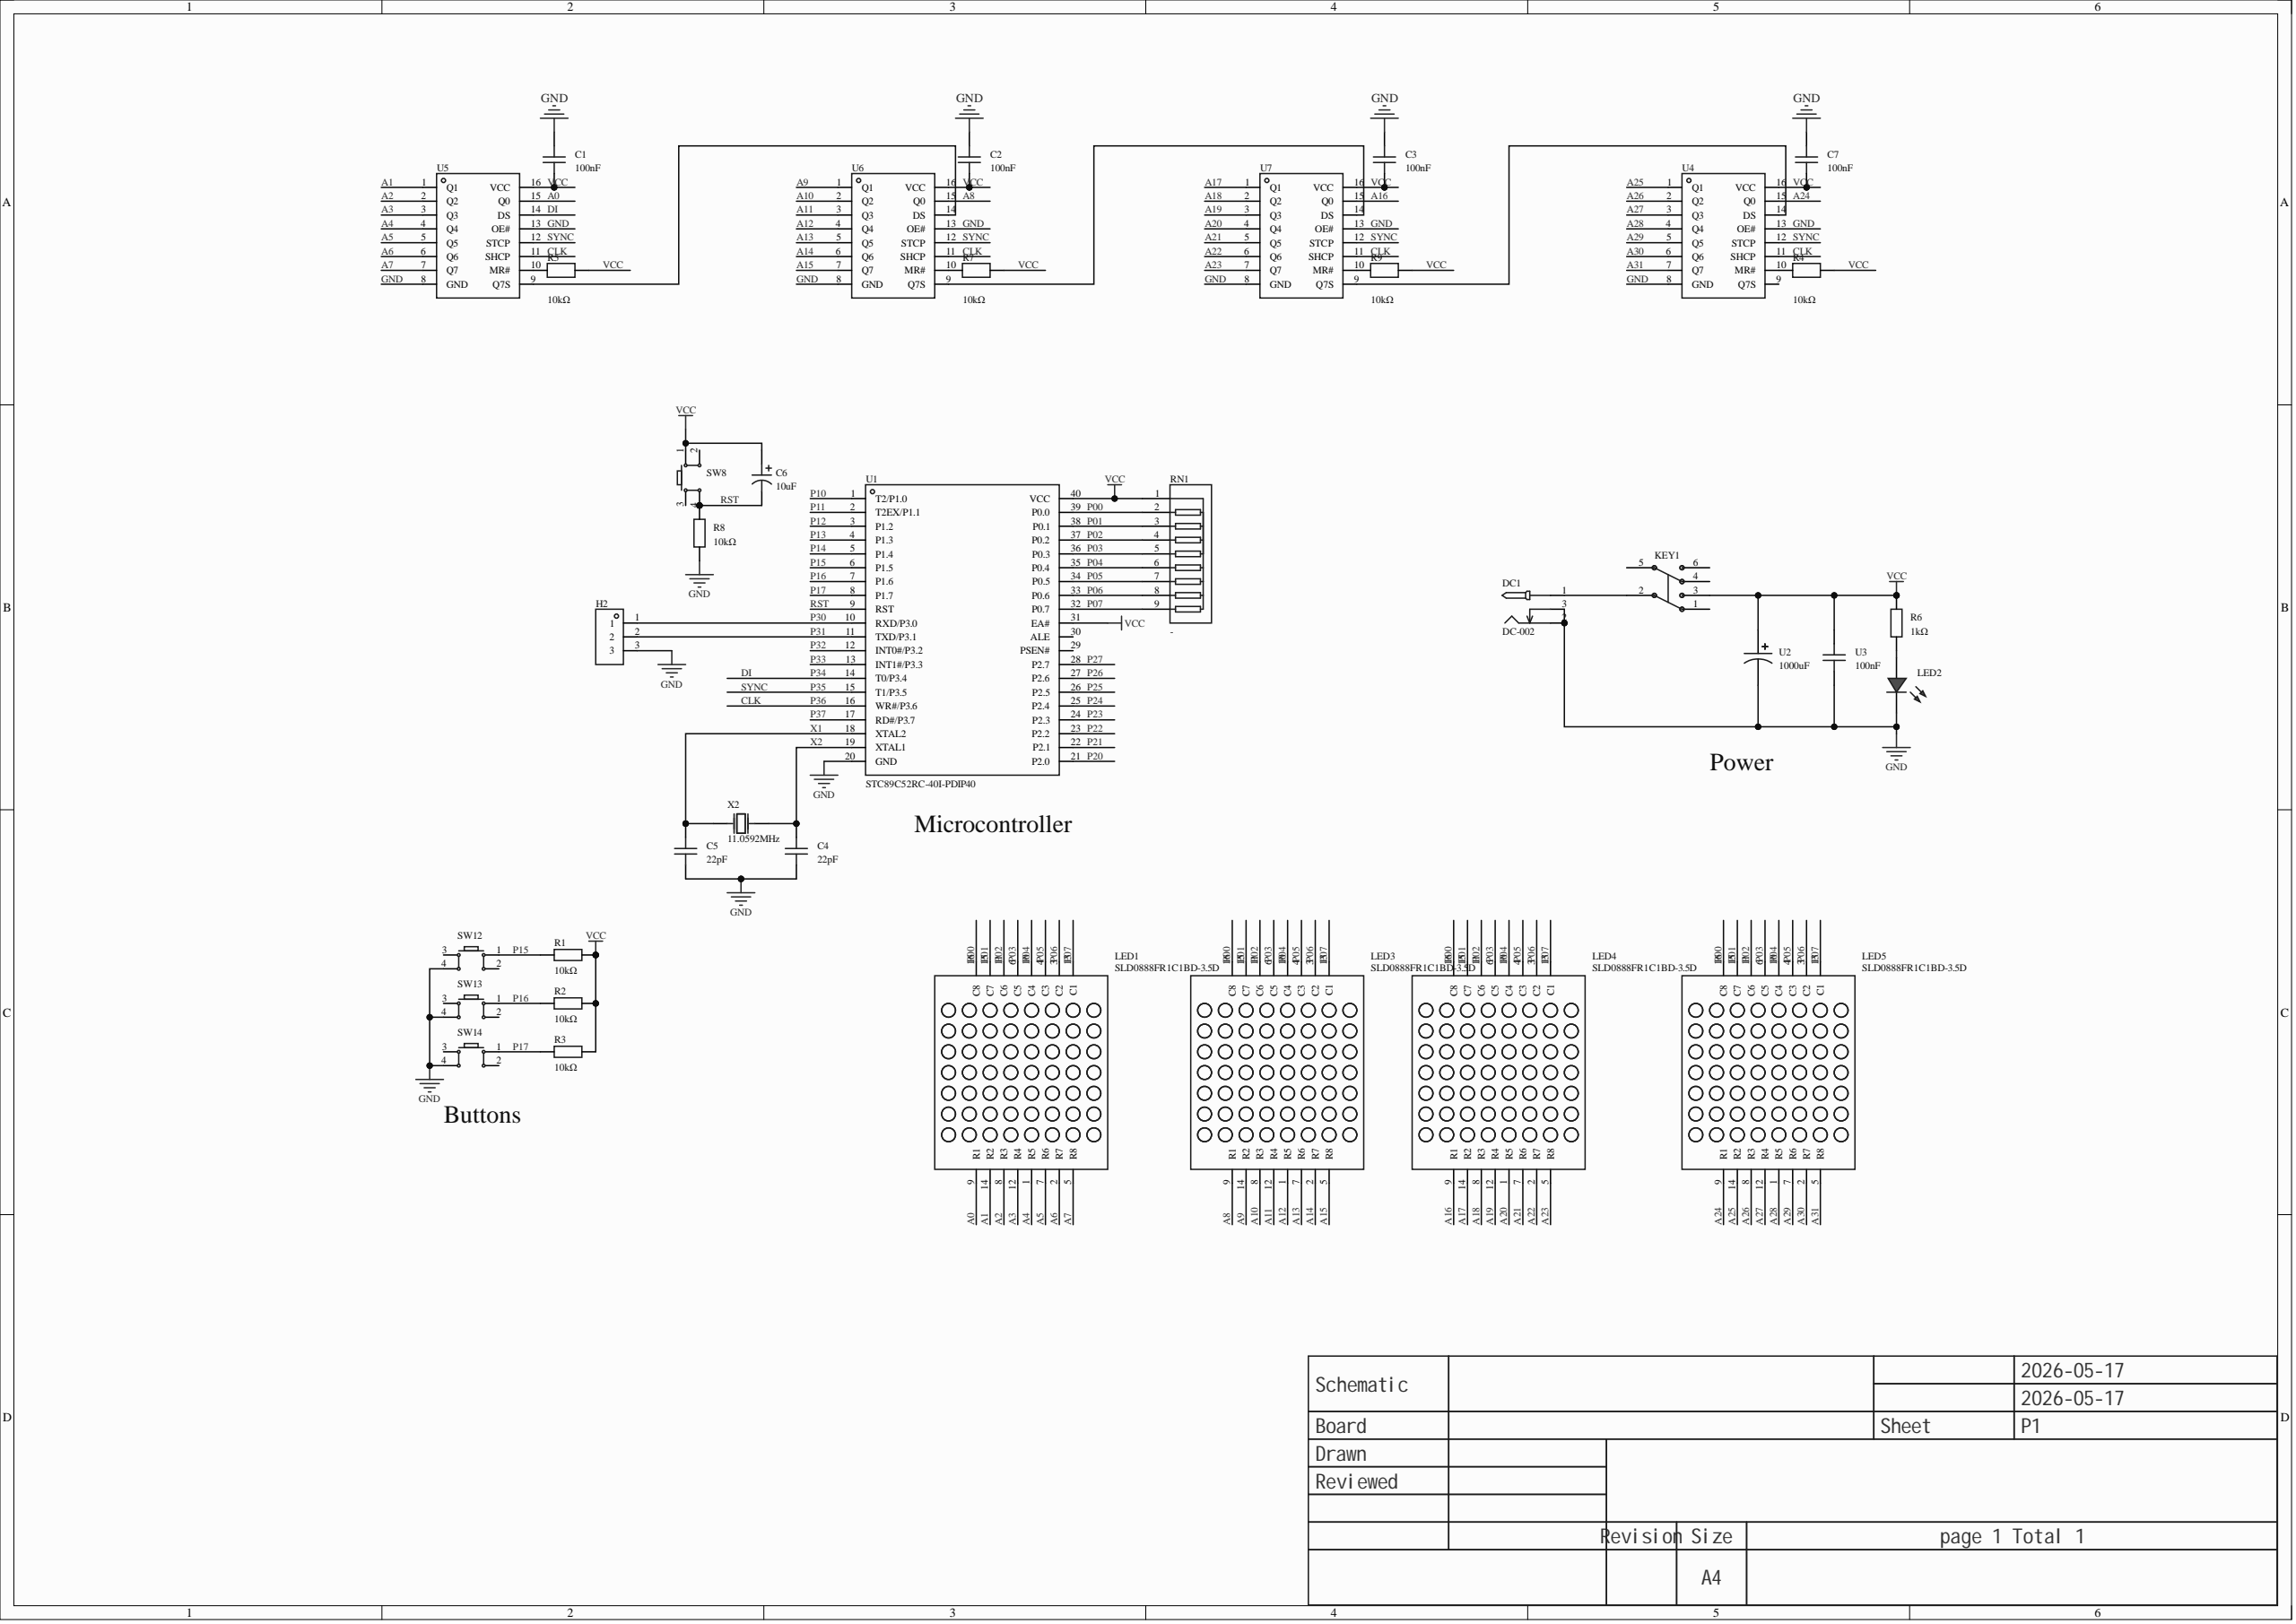Circuit board | Altium Designer | 37 parts | 62 nets
Bill of materials:
Comment,Description,Designator,Footprint,LibRef,Quantity
"100nF","Capacitance: 100nF; tolerance: ±10%; rated voltage: 50V; temperature coefficient: X7R;","C1, C2, C3, C7","C0603","FN18X104K500GBG","4"
"22pF","Capacitance: 30pF; tolerance: ±10%; rated voltage: 25V; temperature coefficient: C0G;","C4, C5","CAP-TH_L3.8-W2.5-P2.54-D0.50","C315C300K3G5TA7301","2"
"10uF","Capacitance: 10uF; tolerance: ±20%; rated voltage: 50V; ripple current: 120mA@100KHz; equivalent series resistance (ESR): 1.6Ω;","C6","CAP-TH_BD5.0-P2.00-D0.8-FD-10UF50VC110GL","10UF50VC110GL","1"
"DC-002","","DC1","DC-IN-TH_DC-3510","DC-002","1"
"","","H2","HDR-TH_3P-P2.54-V-M","HDR-M_2.54_1x3P","1"
"Non-latching switch 8.5×8.5 silent","6 pins, 8.5×8.5","KEY1","SW-TH_6P-L8.5-W8.5-P2.54","无自锁开关 8.5×8.5 无声","1"
"SLD0888FR1C1BD-3.5D","Digits: 8x8; luminous color: red; polarity: common cathode;","LED1, LED3, LED4, LED5","LED-MAT-TH_SLD0888FR1C1BD-3.5D","SLD0888FR1C1BD-3.5D","4"
"","","LED2","LED_TH-3mm","LED_TH-R_3mm","1"
"10kΩ","","R1, R2, R3, R8","Res_1/8W","Res_AXIAL-1/8W","4"
"10kΩ","Resistance: 10kΩ; tolerance: ±5%; power: 62.5mW;","R4, R5, R7, R9","R0402","RCA0210KJLF","4"
"1kΩ","","R6","Res_1/8W","Res_AXIAL-1/8W","1"
"-","Number of resistors: -; resistance: -; power per element: -;","RN1","RES-ARRAY-TH_9P-P2.54-D1.0","排阻 10 K 5%","1"
"","","SW8, SW12, SW13, SW14","SW-TH_4P-L6.0-W6.0-P4.50-LS6.5","Key_TH_6x6x6","4"
"STC89C52RC-40I-PDIP40","CPU core: 51 family; max CPU frequency: -;","U1","DIP-40_L52.0-W13.7-P2.54-LS15.2-BL","STC89C52RC-40I-PDIP40","1"
"1000uF","Capacitance: 1000uF; tolerance: ±20%; rated voltage: 35V; ripple current: 1.18A@120Hz; equivalent series resistance (ESR): -;","U2","CAP-TH_BD12.5-P5.00-D0.6-FD","35YK1000M12.5X20","1"
"100nF","","U3","CAP-TH_L5.0-W2.5-P5.00-D1.0","100nF","1"
"74HC595D,118","Function: serial-to-serial or parallel; supply voltage: 2V~6V; number of elements: 1; bits per element: 8;","U4, U5, U6, U7","SOIC-16_L9.9-W3.9-P1.27-LS6.0-BL","74HC595D,118","4"
"11.059MHz","Crystal type: through-hole crystal; frequency: 11.059MHz; room-temperature tolerance: ±20ppm; load capacitance: 30pF;","X2","OSC-TH_L11.1-W4.7-P4.88","9AC11059302060C3","1"
Netlist (Protel format):
[
C1
C0603
100nF



]
[
C2
C0603
100nF



]
[
C3
C0603
100nF



]
[
C4
CAP-TH_L3.8-W2.5-P2.54-D0.50
22pF



]
[
C5
CAP-TH_L3.8-W2.5-P2.54-D0.50
22pF



]
[
C6
CAP-TH_BD5.0-P2.00-D0.8-FD-10UF50VC110GL
10uF



]
[
C7
C0603
100nF



]
[
DC1
DC-IN-TH_DC-3510
DC-002



]
[
H2
HDR-TH_3P-P2.54-V-M




]
[
KEY1
SW-TH_6P-L8.5-W8.5-P2.54
Non-latching switch 8.5×8.5 silent



]
[
LED1
LED-MAT-TH_SLD0888FR1C1BD-3.5D
SLD0888FR1C1BD-3.5D



]
[
LED2
LED_TH-3mm




]
[
LED3
LED-MAT-TH_SLD0888FR1C1BD-3.5D
SLD0888FR1C1BD-3.5D



]
[
LED4
LED-MAT-TH_SLD0888FR1C1BD-3.5D
SLD0888FR1C1BD-3.5D



]
[
LED5
LED-MAT-TH_SLD0888FR1C1BD-3.5D
SLD0888FR1C1BD-3.5D



]
[
R1
Res_1/8W
10kΩ



]
[
R2
Res_1/8W
10kΩ



]
[
R3
Res_1/8W
10kΩ



]
[
R4
R0402
10kΩ



]
[
R5
R0402
10kΩ



]
[
R6
Res_1/8W
1kΩ



]
[
R7
R0402
10kΩ



]
[
R8
Res_1/8W
10kΩ



]
[
R9
R0402
10kΩ



]
[
RN1
RES-ARRAY-TH_9P-P2.54-D1.0
-



]
[
SW8
SW-TH_4P-L6.0-W6.0-P4.50-LS6.5




]
[
SW12
SW-TH_4P-L6.0-W6.0-P4.50-LS6.5




]
[
SW13
SW-TH_4P-L6.0-W6.0-P4.50-LS6.5




]
[
SW14
SW-TH_4P-L6.0-W6.0-P4.50-LS6.5




]
[
U1
DIP-40_L52.0-W13.7-P2.54-LS15.2-BL
STC89C52RC-40I-PDIP40



]
[
U2
CAP-TH_BD12.5-P5.00-D0.6-FD
1000uF



]
[
U3
CAP-TH_L5.0-W2.5-P5.00-D1.0
100nF



]
[
U4
SOIC-16_L9.9-W3.9-P1.27-LS6.0-BL
74HC595D,118



]
[
U5
SOIC-16_L9.9-W3.9-P1.27-LS6.0-BL
74HC595D,118



]
[
U6
SOIC-16_L9.9-W3.9-P1.27-LS6.0-BL
74HC595D,118



]
[
U7
SOIC-16_L9.9-W3.9-P1.27-LS6.0-BL
74HC595D,118



]
[
X2
OSC-TH_L11.1-W4.7-P4.88
11.0592MHz



]
(
X2
C4-2
U1-19
X2-2
)
(
X1
C5-2
U1-18
X2-1
)
(
VCC
C1-2
C2-2
C3-2
C6-1
C7-2
KEY1-3
R1-2
R2-2
R3-2
R4-2
R5-2
R6-2
R7-2
R9-2
RN1-1
SW8-1
U1-31
U1-40
U2-1
U3-1
U4-16
U5-16
U6-16
U7-16
)
(
RST
C6-2
R8-2
SW8-4
U1-9
)
(
P35
U1-15
U4-12
U5-12
U6-12
U7-12
)
(
P31
H2-2
U1-11
)
(
P30
H2-1
U1-10
)
(
P17
R3-1
SW14-1
U1-8
)
(
P16
R2-1
SW13-1
U1-7
)
(
P15
R1-1
SW12-1
U1-6
)
(
P07
LED1-13
LED3-13
LED4-13
LED5-13
RN1-9
U1-32
)
(
P06
LED1-3
LED3-3
LED4-3
LED5-3
RN1-8
U1-33
)
(
P05
LED1-4
LED3-4
LED4-4
LED5-4
RN1-7
U1-34
)
(
P04
LED1-10
LED3-10
LED4-10
LED5-10
RN1-6
U1-35
)
(
P03
LED1-6
LED3-6
LED4-6
LED5-6
RN1-5
U1-36
)
(
P02
LED1-11
LED3-11
LED4-11
LED5-11
RN1-4
U1-37
)
(
P01
LED1-15
LED3-15
LED4-15
LED5-15
RN1-3
U1-38
)
(
P00
LED1-16
LED3-16
LED4-16
LED5-16
RN1-2
U1-39
)
(
NetU6_9
U6-9
U7-14
)
(
NetU5_9
U5-9
U6-14
)
(
NetU4_14
U4-14
U7-9
)
(
NetR9_1
R9-1
U7-10
)
(
NetR7_1
R7-1
U6-10
)
(
NetR5_1
R5-1
U5-10
)
(
NetR4_1
R4-1
U4-10
)
(
NetLED2_1
LED2-1
R6-1
)
(
NetDC1_1
DC1-1
KEY1-2
)
(
GND
C1-1
C2-1
C3-1
C4-1
C5-1
C7-1
DC1-2
DC1-3
H2-3
LED2-2
R8-1
SW12-4
SW13-4
SW14-4
U1-20
U2-2
U3-2
U4-8
U4-13
U5-8
U5-13
U6-8
U6-13
U7-8
U7-13
)
(
DI
U1-14
U5-14
)
(
CLK
U1-16
U4-11
U5-11
U6-11
U7-11
)
(
A31
LED5-5
U4-7
)
(
A30
LED5-2
U4-6
)
(
A29
LED5-7
U4-5
)
(
A28
LED5-1
U4-4
)
(
A27
LED5-12
U4-3
)
(
A26
LED5-8
U4-2
)
(
A25
LED5-14
U4-1
)
(
A24
LED5-9
U4-15
)
(
A23
LED4-5
U7-7
)
(
A22
LED4-2
U7-6
)
(
A21
LED4-7
U7-5
)
(
A20
LED4-1
U7-4
)
(
A19
LED4-12
U7-3
)
(
A18
LED4-8
U7-2
)
(
A17
LED4-14
U7-1
)
(
A16
LED4-9
U7-15
)
(
A15
LED3-5
U6-7
)
(
A14
LED3-2
U6-6
)
(
A13
LED3-7
U6-5
)
(
A12
LED3-1
U6-4
)
(
A11
LED3-12
U6-3
)
(
A10
LED3-8
U6-2
)
(
A9
LED3-14
U6-1
)
(
A8
LED3-9
U6-15
)
(
A7
LED1-5
U5-7
)
(
A6
LED1-2
U5-6
)
(
A5
LED1-7
U5-5
)
(
A4
LED1-1
U5-4
)
(
A3
LED1-12
U5-3
)
(
A2
LED1-8
U5-2
)
(
A1
LED1-14
U5-1
)
(
A0
LED1-9
U5-15
)